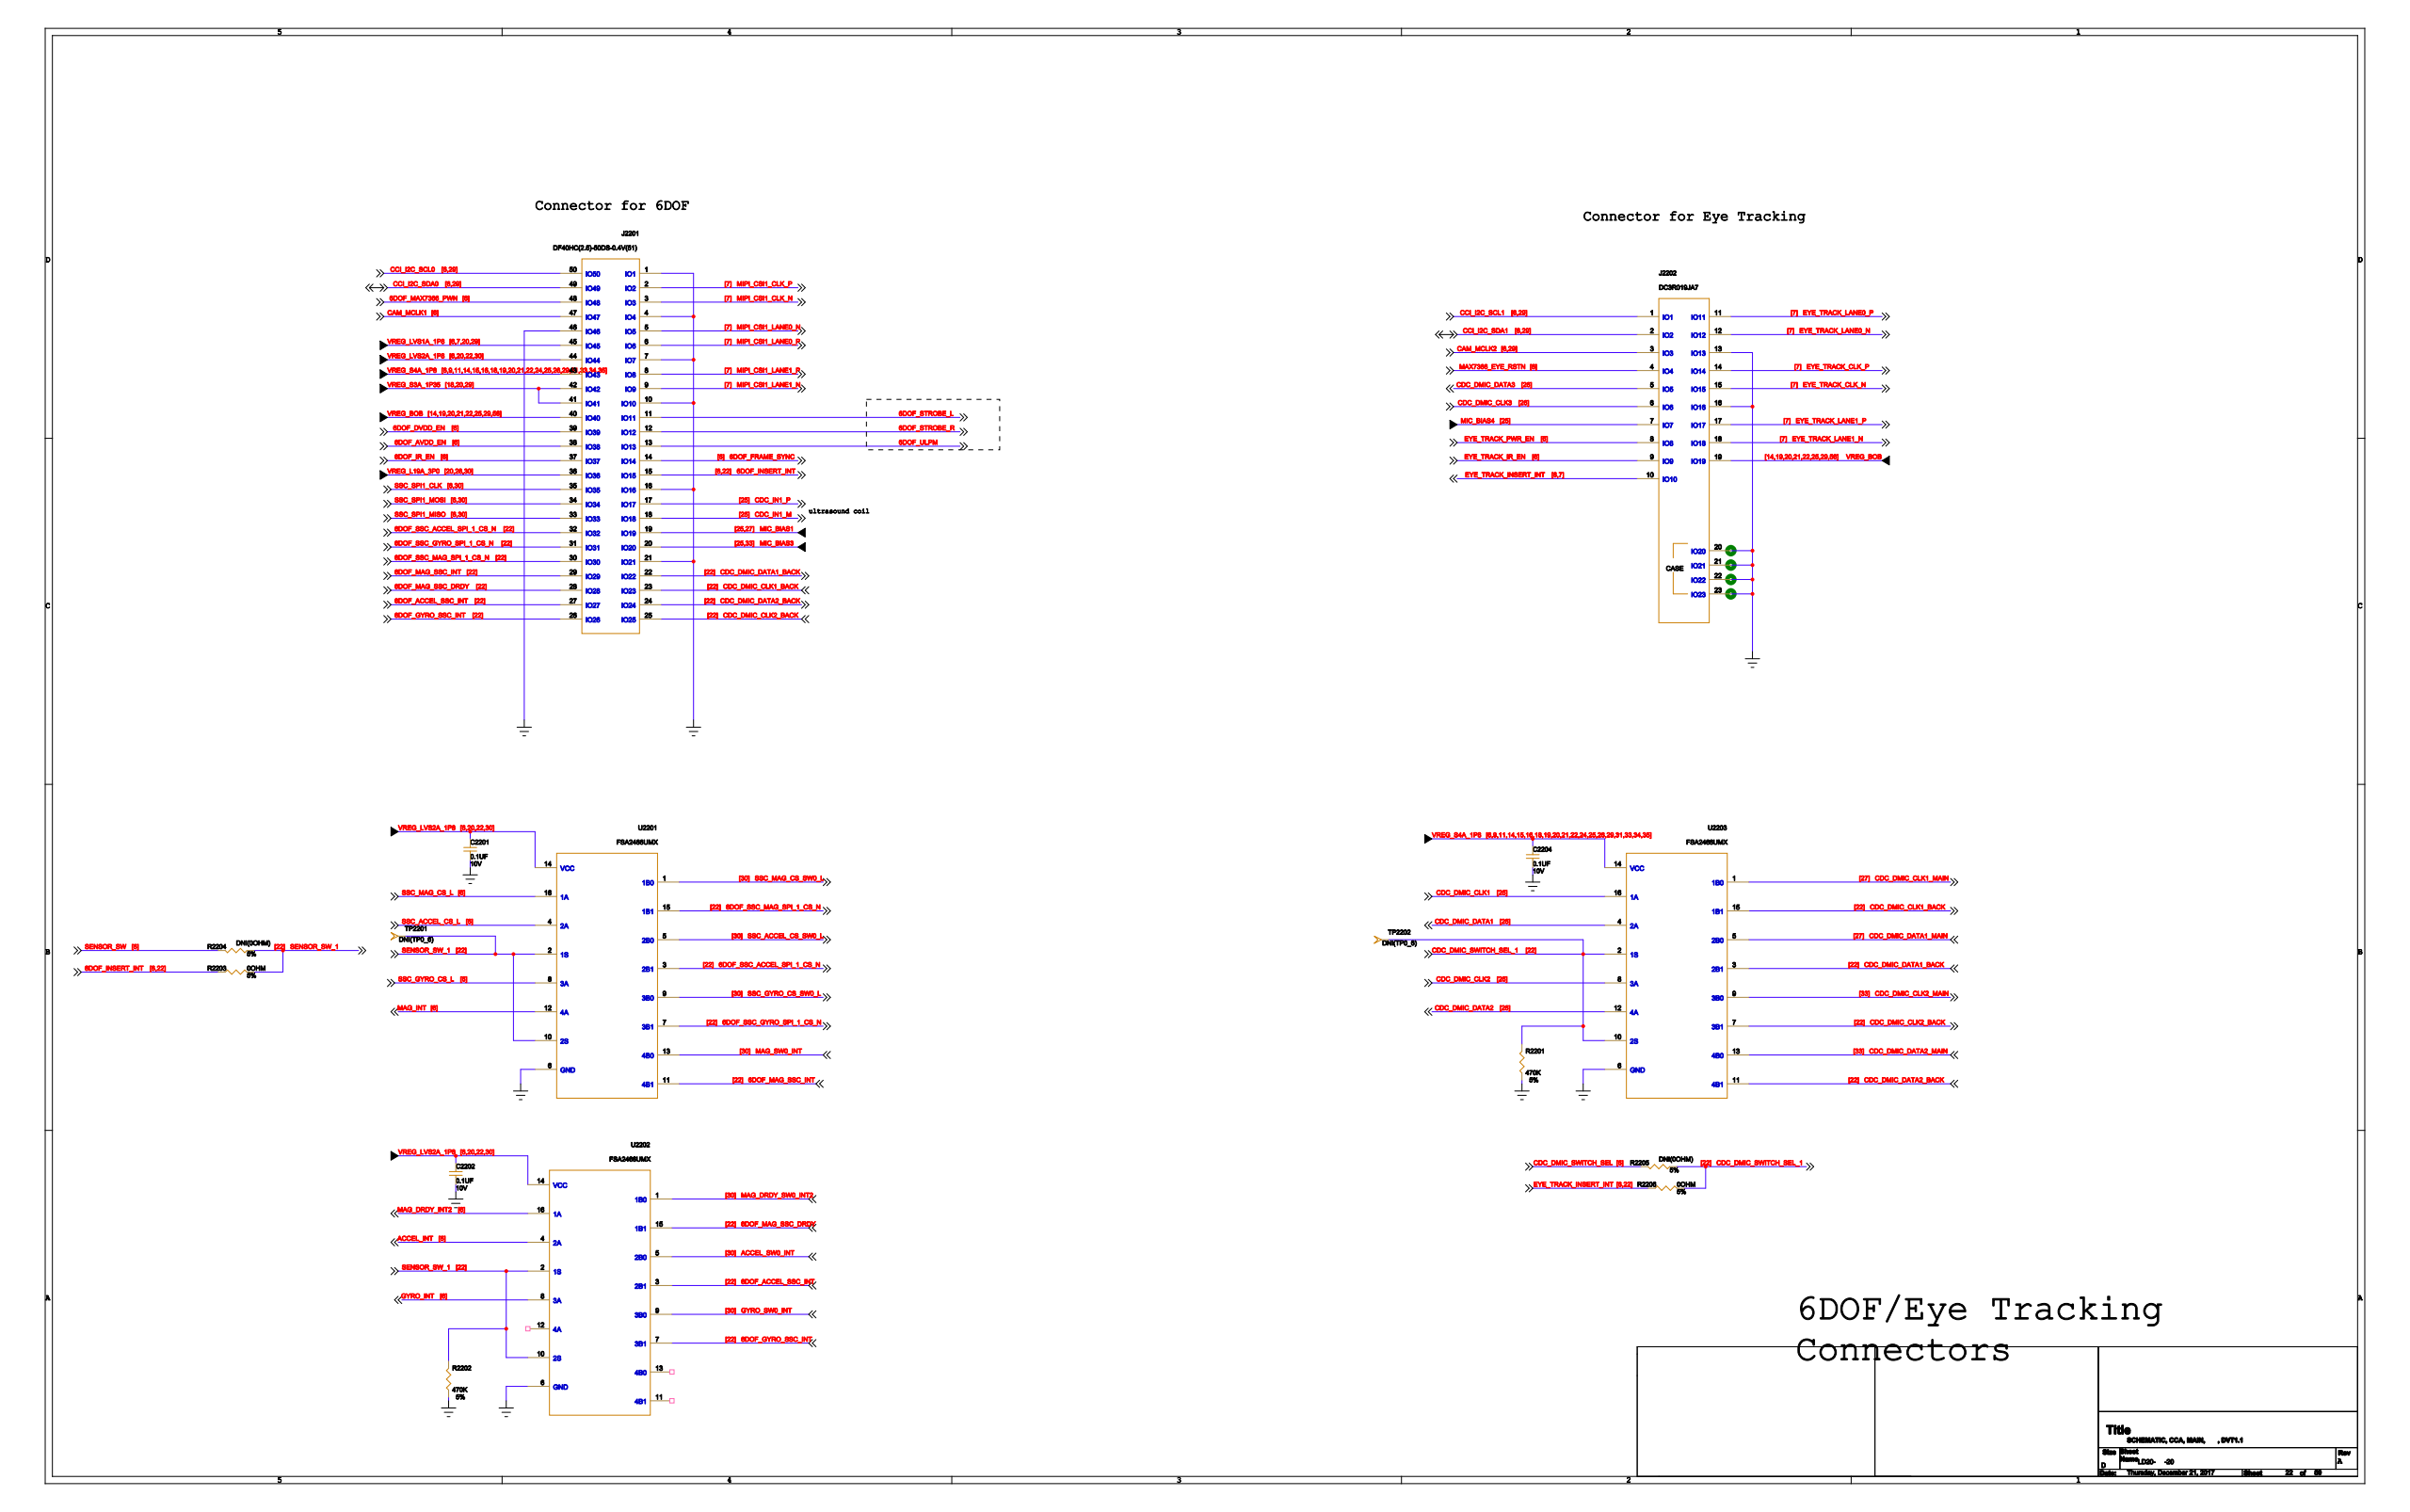Circuit board | Cadence Allegro | 1520 parts | 1149 nets | one sheet of the schematic
Parts on this sheet (reference | value | footprint):
C2201 | 0.1UF | 2P0201R
C2202 | 0.1UF | 2P0201R
C2204 | 0.1UF | 2P0201R
J2201 | DF40HC(2.5)-50DS-0.4V(51) | 50SCONS157V3
J2202 | DC3R019JA7 | 23SCONS157RAV8
R2201 | 470K | 2P0201R
R2202 | 470K | 2P0201R
R2203 | 0OHM | 2P0201R
R2204 | DNI(0OHM) | 2P0201R_DNI
R2205 | DNI(0OHM) | 2P0201R_DNI
R2206 | 0OHM | 2P0201R
TP2201 | DNI(TP0_6) | TP-0_6
TP2202 | DNI(TP0_6) | TP-0_6
U2201 | FSA2466UMX | 16PSM104X73N157
U2202 | FSA2466UMX | 16PSM104X73N157
U2203 | FSA2466UMX | 16PSM104X73N157
Nets of these parts (net: part-pin ...):
GND: C2201-2 C2202-2 C2204-2 R2201-2 R2202-2 U2201-6 U2202-6 U2203-6 J2201-1 J2201-4 J2201-7 J2201-10 J2201-16 J2201-21 J2201-46 J2202-13 J2202-16 J2202-20 J2202-21 J2202-22 J2202-23
VREG_BOB: J2201-40 J2202-19
VREG_S4A_1P8: C2204-1 U2203-14 J2201-43
VREG_L19A_3P0: J2201-36
VREG_LVS2A_1P8: C2201-1 C2202-1 U2201-14 U2202-14 J2201-44
CCI_I2C_SCL1: J2202-1
EYE_TRACK_INSERT_INT: R2206-2 J2202-10
EYE_TRACK_LANE0_P: J2202-11
EYE_TRACK_LANE0_N: J2202-12
EYE_TRACK_CLK_P: J2202-14
EYE_TRACK_CLK_N: J2202-15
EYE_TRACK_LANE1_P: J2202-17
EYE_TRACK_LANE1_N: J2202-18
CCI_I2C_SDA1: J2202-2
CAM_MCLK2: J2202-3
MAX7366_EYE_RSTN: J2202-4
CDC_DMIC_DATA3: J2202-5
CDC_DMIC_CLK3: J2202-6
MIC_BIAS4: J2202-7
EYE_TRACK_PWR_EN: J2202-8
EYE_TRACK_IR_EN: J2202-9
6DOF_STROBE_L: J2201-11
6DOF_STROBE_R: J2201-12
6DOF_ULPM: J2201-13
6DOF_FRAME_SYNC: J2201-14
6DOF_INSERT_INT: R2203-2 J2201-15
CDC_IN1_P: J2201-17
CDC_IN1_M: J2201-18
MIC_BIAS1: J2201-19
MIPI_CSI1_CLK_P: J2201-2
MIC_BIAS3: J2201-20
CDC_DMIC_DATA1_BACK: U2203-3 J2201-22
CDC_DMIC_CLK1_BACK: U2203-15 J2201-23
CDC_DMIC_DATA2_BACK: U2203-11 J2201-24
CDC_DMIC_CLK2_BACK: U2203-7 J2201-25
6DOF_GYRO_SSC_INT: U2202-7 J2201-26
6DOF_ACCEL_SSC_INT: U2202-3 J2201-27
6DOF_MAG_SSC_DRDY: U2202-15 J2201-28
6DOF_MAG_SSC_INT: U2201-11 J2201-29
MIPI_CSI1_CLK_N: J2201-3
6DOF_SSC_MAG_SPI_1_CS_N: U2201-15 J2201-30
6DOF_SSC_GYRO_SPI_1_CS_N: U2201-7 J2201-31
6DOF_SSC_ACCEL_SPI_1_CS_N: U2201-3 J2201-32
SSC_SPI1_MISO: J2201-33
SSC_SPI1_MOSI: J2201-34
SSC_SPI1_CLK: J2201-35
6DOF_IR_EN: J2201-37
6DOF_AVDD_EN: J2201-38
6DOF_DVDD_EN: J2201-39
VREG_S3A_1P35: J2201-41 J2201-42
VREG_LVS1A_1P8: J2201-45
CAM_MCLK1: J2201-47
6DOF_MAX7366_PWN: J2201-48
CCI_I2C_SDA0: J2201-49
MIPI_CSI1_LANE0_N: J2201-5
CCI_I2C_SCL0: J2201-50
MIPI_CSI1_LANE0_P: J2201-6
MIPI_CSI1_LANE1_P: J2201-8
MIPI_CSI1_LANE1_N: J2201-9
CDC_DMIC_SWITCH_SEL_1: R2201-1 R2205-2 R2206-1 TP2202-1 U2203-2 U2203-10
SENSOR_SW_1: R2202-1 R2203-1 R2204-2 TP2201-1 U2201-2 U2201-10 U2202-2 U2202-10
CDC_DMIC_CLK1_MAIN: U2203-1
CDC_DMIC_DATA1_MAIN: U2203-5
CDC_DMIC_CLK1: U2203-16
CDC_DMIC_DATA1: U2203-4
CDC_DMIC_CLK2: U2203-8
CDC_DMIC_CLK2_MAIN: U2203-9
CDC_DMIC_DATA2: U2203-12
CDC_DMIC_DATA2_MAIN: U2203-13
SSC_MAG_CS_L: U2201-16
SSC_MAG_CS_SW0_L: U2201-1
SSC_ACCEL_CS_L: U2201-4
SSC_ACCEL_CS_SW0_L: U2201-5
SSC_GYRO_CS_L: U2201-8
SSC_GYRO_CS_SW0_L: U2201-9
MAG_INT: U2201-12
MAG_SW0_INT: U2201-13
MAG_DRDY_INT2: U2202-16
MAG_DRDY_SW0_INT2: U2202-1
ACCEL_INT: U2202-4
ACCEL_SW0_INT: U2202-5
GYRO_INT: U2202-8
GYRO_SW0_INT: U2202-9
SENSOR_SW: R2204-1
CDC_DMIC_SWITCH_SEL: R2205-1